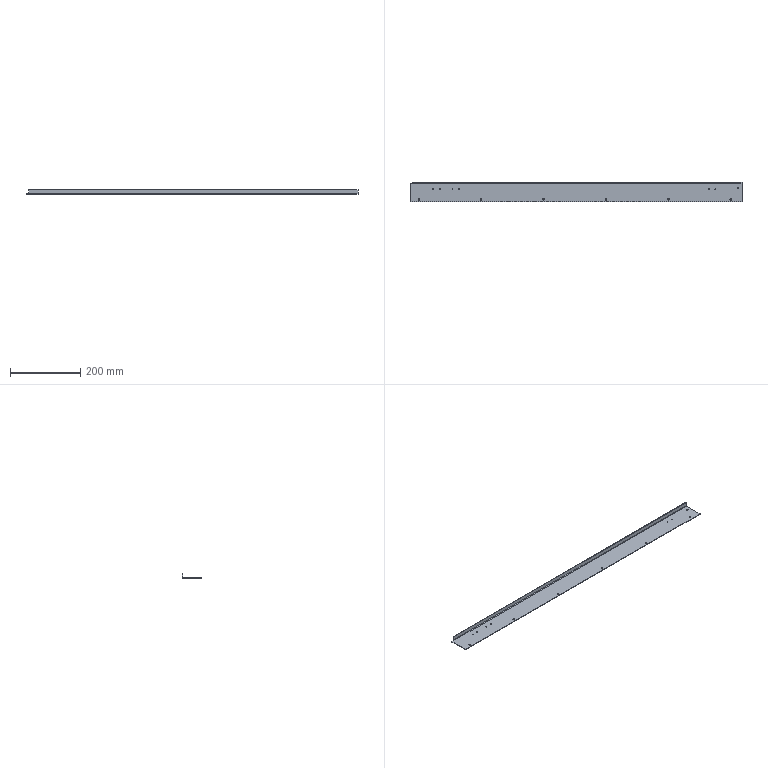Part | STEP file | 866-BDO024-95-04A | 1 solid | 38 faces | box 942 x 56.5 x 13.5 mm | volume 95046 mm3 | cylinder 28 | plane 10 | commonest cylinder face diameters 4.5 x14 2.5 x12 3 x1 6 x1
STEP:
#1=CARTESIAN_POINT('',(730.75,7.5,0.));
#2=VERTEX_POINT('',#1);
#3=CARTESIAN_POINT('',(735.25,7.5,0.));
#4=VERTEX_POINT('',#3);
#5=CARTESIAN_POINT('',(733.,7.5,0.));
#6=DIRECTION('',(0.,0.,1.));
#7=DIRECTION('',(1.,0.,0.));
#8=AXIS2_PLACEMENT_3D('',#5,#6,#7);
#9=CIRCLE('',#8,2.25);
#10=EDGE_CURVE('',#2,#4,#9,.T.);
#11=ORIENTED_EDGE('',*,*,#10,.F.);
#12=CARTESIAN_POINT('',(730.75,7.5,1.5));
#13=VERTEX_POINT('',#12);
#14=CARTESIAN_POINT('',(730.75,7.5,1.5));
#15=DIRECTION('',(0.,0.,1.));
#16=VECTOR('',#15,1000.);
#17=LINE('',#14,#16);
#18=EDGE_CURVE('',#2,#13,#17,.T.);
#19=ORIENTED_EDGE('',*,*,#18,.T.);
#20=CARTESIAN_POINT('',(735.25,7.5,1.5));
#21=VERTEX_POINT('',#20);
#22=CARTESIAN_POINT('',(733.,7.5,1.5));
#23=DIRECTION('',(0.,0.,-1.));
#24=DIRECTION('',(1.,0.,0.));
#25=AXIS2_PLACEMENT_3D('',#22,#23,#24);
#26=CIRCLE('',#25,2.25);
#27=EDGE_CURVE('',#21,#13,#26,.T.);
#28=ORIENTED_EDGE('',*,*,#27,.F.);
#29=CARTESIAN_POINT('',(735.25,7.5,1.5));
#30=DIRECTION('',(0.,0.,1.));
#31=VECTOR('',#30,1000.);
#32=LINE('',#29,#31);
#33=EDGE_CURVE('',#4,#21,#32,.T.);
#34=ORIENTED_EDGE('',*,*,#33,.F.);
#35=EDGE_LOOP('',(#11,#19,#28,#34));
#36=FACE_OUTER_BOUND('',#35,.T.);
#37=CARTESIAN_POINT('',(733.,7.5,1.5));
#38=DIRECTION('',(0.,0.,1.));
#39=DIRECTION('',(1.,0.,0.));
#40=AXIS2_PLACEMENT_3D('',#37,#38,#39);
#41=CYLINDRICAL_SURFACE('',#40,2.25);
#42=ADVANCED_FACE('',(#36),#41,.F.);
#43=CARTESIAN_POINT('',(199.75,7.5,0.));
#44=VERTEX_POINT('',#43);
#45=CARTESIAN_POINT('',(204.25,7.5,0.));
#46=VERTEX_POINT('',#45);
#47=CARTESIAN_POINT('',(202.,7.5,0.));
#48=DIRECTION('',(0.,0.,1.));
#49=DIRECTION('',(1.,0.,0.));
#50=AXIS2_PLACEMENT_3D('',#47,#48,#49);
#51=CIRCLE('',#50,2.25);
#52=EDGE_CURVE('',#44,#46,#51,.T.);
#53=ORIENTED_EDGE('',*,*,#52,.F.);
#54=CARTESIAN_POINT('',(199.75,7.5,1.5));
#55=VERTEX_POINT('',#54);
#56=CARTESIAN_POINT('',(199.75,7.5,1.5));
#57=DIRECTION('',(0.,0.,1.));
#58=VECTOR('',#57,1000.);
#59=LINE('',#56,#58);
#60=EDGE_CURVE('',#44,#55,#59,.T.);
#61=ORIENTED_EDGE('',*,*,#60,.T.);
#62=CARTESIAN_POINT('',(204.25,7.5,1.5));
#63=VERTEX_POINT('',#62);
#64=CARTESIAN_POINT('',(202.,7.5,1.5));
#65=DIRECTION('',(0.,0.,-1.));
#66=DIRECTION('',(1.,0.,0.));
#67=AXIS2_PLACEMENT_3D('',#64,#65,#66);
#68=CIRCLE('',#67,2.25);
#69=EDGE_CURVE('',#63,#55,#68,.T.);
#70=ORIENTED_EDGE('',*,*,#69,.F.);
#71=CARTESIAN_POINT('',(204.25,7.5,1.5));
#72=DIRECTION('',(0.,0.,1.));
#73=VECTOR('',#72,1000.);
#74=LINE('',#71,#73);
#75=EDGE_CURVE('',#46,#63,#74,.T.);
#76=ORIENTED_EDGE('',*,*,#75,.F.);
#77=EDGE_LOOP('',(#53,#61,#70,#76));
#78=FACE_OUTER_BOUND('',#77,.T.);
#79=CARTESIAN_POINT('',(202.,7.5,1.5));
#80=DIRECTION('',(0.,0.,1.));
#81=DIRECTION('',(1.,0.,0.));
#82=AXIS2_PLACEMENT_3D('',#79,#80,#81);
#83=CYLINDRICAL_SURFACE('',#82,2.25);
#84=ADVANCED_FACE('',(#78),#83,.F.);
#85=CARTESIAN_POINT('',(376.75,7.5,0.));
#86=VERTEX_POINT('',#85);
#87=CARTESIAN_POINT('',(381.25,7.5,0.));
#88=VERTEX_POINT('',#87);
#89=CARTESIAN_POINT('',(379.,7.5,0.));
#90=DIRECTION('',(0.,0.,1.));
#91=DIRECTION('',(1.,0.,0.));
#92=AXIS2_PLACEMENT_3D('',#89,#90,#91);
#93=CIRCLE('',#92,2.25);
#94=EDGE_CURVE('',#86,#88,#93,.T.);
#95=ORIENTED_EDGE('',*,*,#94,.F.);
#96=CARTESIAN_POINT('',(376.75,7.5,1.5));
#97=VERTEX_POINT('',#96);
#98=CARTESIAN_POINT('',(376.75,7.5,1.5));
#99=DIRECTION('',(0.,0.,1.));
#100=VECTOR('',#99,1000.);
#101=LINE('',#98,#100);
#102=EDGE_CURVE('',#86,#97,#101,.T.);
#103=ORIENTED_EDGE('',*,*,#102,.T.);
#104=CARTESIAN_POINT('',(381.25,7.5,1.5));
#105=VERTEX_POINT('',#104);
#106=CARTESIAN_POINT('',(379.,7.5,1.5));
#107=DIRECTION('',(0.,0.,-1.));
#108=DIRECTION('',(1.,0.,0.));
#109=AXIS2_PLACEMENT_3D('',#106,#107,#108);
#110=CIRCLE('',#109,2.25);
#111=EDGE_CURVE('',#105,#97,#110,.T.);
#112=ORIENTED_EDGE('',*,*,#111,.F.);
#113=CARTESIAN_POINT('',(381.25,7.5,1.5));
#114=DIRECTION('',(0.,0.,1.));
#115=VECTOR('',#114,1000.);
#116=LINE('',#113,#115);
#117=EDGE_CURVE('',#88,#105,#116,.T.);
#118=ORIENTED_EDGE('',*,*,#117,.F.);
#119=EDGE_LOOP('',(#95,#103,#112,#118));
#120=FACE_OUTER_BOUND('',#119,.T.);
#121=CARTESIAN_POINT('',(379.,7.5,1.5));
#122=DIRECTION('',(0.,0.,1.));
#123=DIRECTION('',(1.,0.,0.));
#124=AXIS2_PLACEMENT_3D('',#121,#122,#123);
#125=CYLINDRICAL_SURFACE('',#124,2.25);
#126=ADVANCED_FACE('',(#120),#125,.F.);
#127=CARTESIAN_POINT('',(553.75,7.5,0.));
#128=VERTEX_POINT('',#127);
#129=CARTESIAN_POINT('',(558.25,7.5,0.));
#130=VERTEX_POINT('',#129);
#131=CARTESIAN_POINT('',(556.,7.5,0.));
#132=DIRECTION('',(0.,0.,1.));
#133=DIRECTION('',(1.,0.,0.));
#134=AXIS2_PLACEMENT_3D('',#131,#132,#133);
#135=CIRCLE('',#134,2.25);
#136=EDGE_CURVE('',#128,#130,#135,.T.);
#137=ORIENTED_EDGE('',*,*,#136,.F.);
#138=CARTESIAN_POINT('',(553.75,7.5,1.5));
#139=VERTEX_POINT('',#138);
#140=CARTESIAN_POINT('',(553.75,7.5,1.5));
#141=DIRECTION('',(0.,0.,1.));
#142=VECTOR('',#141,1000.);
#143=LINE('',#140,#142);
#144=EDGE_CURVE('',#128,#139,#143,.T.);
#145=ORIENTED_EDGE('',*,*,#144,.T.);
#146=CARTESIAN_POINT('',(558.25,7.5,1.5));
#147=VERTEX_POINT('',#146);
#148=CARTESIAN_POINT('',(556.,7.5,1.5));
#149=DIRECTION('',(0.,0.,-1.));
#150=DIRECTION('',(1.,0.,0.));
#151=AXIS2_PLACEMENT_3D('',#148,#149,#150);
#152=CIRCLE('',#151,2.25);
#153=EDGE_CURVE('',#147,#139,#152,.T.);
#154=ORIENTED_EDGE('',*,*,#153,.F.);
#155=CARTESIAN_POINT('',(558.25,7.5,1.5));
#156=DIRECTION('',(0.,0.,1.));
#157=VECTOR('',#156,1000.);
#158=LINE('',#155,#157);
#159=EDGE_CURVE('',#130,#147,#158,.T.);
#160=ORIENTED_EDGE('',*,*,#159,.F.);
#161=EDGE_LOOP('',(#137,#145,#154,#160));
#162=FACE_OUTER_BOUND('',#161,.T.);
#163=CARTESIAN_POINT('',(556.,7.5,1.5));
#164=DIRECTION('',(0.,0.,1.));
#165=DIRECTION('',(1.,0.,0.));
#166=AXIS2_PLACEMENT_3D('',#163,#164,#165);
#167=CYLINDRICAL_SURFACE('',#166,2.25);
#168=ADVANCED_FACE('',(#162),#167,.F.);
#169=CARTESIAN_POINT('',(928.25,40.,0.));
#170=VERTEX_POINT('',#169);
#171=CARTESIAN_POINT('',(932.75,40.,0.));
#172=VERTEX_POINT('',#171);
#173=CARTESIAN_POINT('',(930.5,40.,0.));
#174=DIRECTION('',(0.,0.,1.));
#175=DIRECTION('',(1.,0.,0.));
#176=AXIS2_PLACEMENT_3D('',#173,#174,#175);
#177=CIRCLE('',#176,2.25);
#178=EDGE_CURVE('',#170,#172,#177,.T.);
#179=ORIENTED_EDGE('',*,*,#178,.F.);
#180=CARTESIAN_POINT('',(928.25,40.,1.5));
#181=VERTEX_POINT('',#180);
#182=CARTESIAN_POINT('',(928.25,40.,1.5));
#183=DIRECTION('',(0.,0.,1.));
#184=VECTOR('',#183,1000.);
#185=LINE('',#182,#184);
#186=EDGE_CURVE('',#170,#181,#185,.T.);
#187=ORIENTED_EDGE('',*,*,#186,.T.);
#188=CARTESIAN_POINT('',(932.75,40.,1.5));
#189=VERTEX_POINT('',#188);
#190=CARTESIAN_POINT('',(930.5,40.,1.5));
#191=DIRECTION('',(0.,0.,-1.));
#192=DIRECTION('',(1.,0.,0.));
#193=AXIS2_PLACEMENT_3D('',#190,#191,#192);
#194=CIRCLE('',#193,2.25);
#195=EDGE_CURVE('',#189,#181,#194,.T.);
#196=ORIENTED_EDGE('',*,*,#195,.F.);
#197=CARTESIAN_POINT('',(932.75,40.,1.5));
#198=DIRECTION('',(0.,0.,1.));
#199=VECTOR('',#198,1000.);
#200=LINE('',#197,#199);
#201=EDGE_CURVE('',#172,#189,#200,.T.);
#202=ORIENTED_EDGE('',*,*,#201,.F.);
#203=EDGE_LOOP('',(#179,#187,#196,#202));
#204=FACE_OUTER_BOUND('',#203,.T.);
#205=CARTESIAN_POINT('',(930.5,40.,1.5));
#206=DIRECTION('',(0.,0.,1.));
#207=DIRECTION('',(1.,0.,0.));
#208=AXIS2_PLACEMENT_3D('',#205,#206,#207);
#209=CYLINDRICAL_SURFACE('',#208,2.25);
#210=ADVANCED_FACE('',(#204),#209,.F.);
#211=CARTESIAN_POINT('',(907.75,7.5,0.));
#212=VERTEX_POINT('',#211);
#213=CARTESIAN_POINT('',(912.25,7.5,0.));
#214=VERTEX_POINT('',#213);
#215=CARTESIAN_POINT('',(910.,7.5,0.));
#216=DIRECTION('',(0.,0.,1.));
#217=DIRECTION('',(1.,0.,0.));
#218=AXIS2_PLACEMENT_3D('',#215,#216,#217);
#219=CIRCLE('',#218,2.25);
#220=EDGE_CURVE('',#212,#214,#219,.T.);
#221=ORIENTED_EDGE('',*,*,#220,.F.);
#222=CARTESIAN_POINT('',(907.75,7.5,1.5));
#223=VERTEX_POINT('',#222);
#224=CARTESIAN_POINT('',(907.75,7.5,1.5));
#225=DIRECTION('',(0.,0.,1.));
#226=VECTOR('',#225,1000.);
#227=LINE('',#224,#226);
#228=EDGE_CURVE('',#212,#223,#227,.T.);
#229=ORIENTED_EDGE('',*,*,#228,.T.);
#230=CARTESIAN_POINT('',(912.25,7.5,1.5));
#231=VERTEX_POINT('',#230);
#232=CARTESIAN_POINT('',(910.,7.5,1.5));
#233=DIRECTION('',(0.,0.,-1.));
#234=DIRECTION('',(1.,0.,0.));
#235=AXIS2_PLACEMENT_3D('',#232,#233,#234);
#236=CIRCLE('',#235,2.25);
#237=EDGE_CURVE('',#231,#223,#236,.T.);
#238=ORIENTED_EDGE('',*,*,#237,.F.);
#239=CARTESIAN_POINT('',(912.25,7.5,1.5));
#240=DIRECTION('',(0.,0.,1.));
#241=VECTOR('',#240,1000.);
#242=LINE('',#239,#241);
#243=EDGE_CURVE('',#214,#231,#242,.T.);
#244=ORIENTED_EDGE('',*,*,#243,.F.);
#245=EDGE_LOOP('',(#221,#229,#238,#244));
#246=FACE_OUTER_BOUND('',#245,.T.);
#247=CARTESIAN_POINT('',(910.,7.5,1.5));
#248=DIRECTION('',(0.,0.,1.));
#249=DIRECTION('',(1.,0.,0.));
#250=AXIS2_PLACEMENT_3D('',#247,#248,#249);
#251=CYLINDRICAL_SURFACE('',#250,2.25);
#252=ADVANCED_FACE('',(#246),#251,.F.);
#253=CARTESIAN_POINT('',(22.75,7.5,0.));
#254=VERTEX_POINT('',#253);
#255=CARTESIAN_POINT('',(27.25,7.5,0.));
#256=VERTEX_POINT('',#255);
#257=CARTESIAN_POINT('',(25.,7.5,0.));
#258=DIRECTION('',(0.,0.,1.));
#259=DIRECTION('',(1.,0.,0.));
#260=AXIS2_PLACEMENT_3D('',#257,#258,#259);
#261=CIRCLE('',#260,2.25);
#262=EDGE_CURVE('',#254,#256,#261,.T.);
#263=ORIENTED_EDGE('',*,*,#262,.F.);
#264=CARTESIAN_POINT('',(22.75,7.5,1.5));
#265=VERTEX_POINT('',#264);
#266=CARTESIAN_POINT('',(22.75,7.5,1.5));
#267=DIRECTION('',(0.,0.,1.));
#268=VECTOR('',#267,1000.);
#269=LINE('',#266,#268);
#270=EDGE_CURVE('',#254,#265,#269,.T.);
#271=ORIENTED_EDGE('',*,*,#270,.T.);
#272=CARTESIAN_POINT('',(27.25,7.5,1.5));
#273=VERTEX_POINT('',#272);
#274=CARTESIAN_POINT('',(25.,7.5,1.5));
#275=DIRECTION('',(0.,0.,-1.));
#276=DIRECTION('',(1.,0.,0.));
#277=AXIS2_PLACEMENT_3D('',#274,#275,#276);
#278=CIRCLE('',#277,2.25);
#279=EDGE_CURVE('',#273,#265,#278,.T.);
#280=ORIENTED_EDGE('',*,*,#279,.F.);
#281=CARTESIAN_POINT('',(27.25,7.5,1.5));
#282=DIRECTION('',(0.,0.,1.));
#283=VECTOR('',#282,1000.);
#284=LINE('',#281,#283);
#285=EDGE_CURVE('',#256,#273,#284,.T.);
#286=ORIENTED_EDGE('',*,*,#285,.F.);
#287=EDGE_LOOP('',(#263,#271,#280,#286));
#288=FACE_OUTER_BOUND('',#287,.T.);
#289=CARTESIAN_POINT('',(25.,7.5,1.5));
#290=DIRECTION('',(0.,0.,1.));
#291=DIRECTION('',(1.,0.,0.));
#292=AXIS2_PLACEMENT_3D('',#289,#290,#291);
#293=CYLINDRICAL_SURFACE('',#292,2.25);
#294=ADVANCED_FACE('',(#288),#293,.F.);
#295=CARTESIAN_POINT('',(865.25,36.,0.));
#296=VERTEX_POINT('',#295);
#297=CARTESIAN_POINT('',(867.75,36.,0.));
#298=VERTEX_POINT('',#297);
#299=CARTESIAN_POINT('',(866.5,36.,0.));
#300=DIRECTION('',(0.,0.,1.));
#301=DIRECTION('',(1.,0.,0.));
#302=AXIS2_PLACEMENT_3D('',#299,#300,#301);
#303=CIRCLE('',#302,1.25);
#304=EDGE_CURVE('',#296,#298,#303,.T.);
#305=ORIENTED_EDGE('',*,*,#304,.F.);
#306=CARTESIAN_POINT('',(865.25,36.,1.5));
#307=VERTEX_POINT('',#306);
#308=CARTESIAN_POINT('',(865.25,36.,1.5));
#309=DIRECTION('',(0.,0.,1.));
#310=VECTOR('',#309,1000.);
#311=LINE('',#308,#310);
#312=EDGE_CURVE('',#296,#307,#311,.T.);
#313=ORIENTED_EDGE('',*,*,#312,.T.);
#314=CARTESIAN_POINT('',(867.75,36.,1.5));
#315=VERTEX_POINT('',#314);
#316=CARTESIAN_POINT('',(866.5,36.,1.5));
#317=DIRECTION('',(0.,0.,-1.));
#318=DIRECTION('',(1.,0.,0.));
#319=AXIS2_PLACEMENT_3D('',#316,#317,#318);
#320=CIRCLE('',#319,1.25);
#321=EDGE_CURVE('',#315,#307,#320,.T.);
#322=ORIENTED_EDGE('',*,*,#321,.F.);
#323=CARTESIAN_POINT('',(867.75,36.,1.5));
#324=DIRECTION('',(0.,0.,1.));
#325=VECTOR('',#324,1000.);
#326=LINE('',#323,#325);
#327=EDGE_CURVE('',#298,#315,#326,.T.);
#328=ORIENTED_EDGE('',*,*,#327,.F.);
#329=EDGE_LOOP('',(#305,#313,#322,#328));
#330=FACE_OUTER_BOUND('',#329,.T.);
#331=CARTESIAN_POINT('',(866.5,36.,1.5));
#332=DIRECTION('',(0.,0.,1.));
#333=DIRECTION('',(1.,0.,0.));
#334=AXIS2_PLACEMENT_3D('',#331,#332,#333);
#335=CYLINDRICAL_SURFACE('',#334,1.25);
#336=ADVANCED_FACE('',(#330),#335,.F.);
#337=CARTESIAN_POINT('',(846.25,36.,0.));
#338=VERTEX_POINT('',#337);
#339=CARTESIAN_POINT('',(848.75,36.,0.));
#340=VERTEX_POINT('',#339);
#341=CARTESIAN_POINT('',(847.5,36.,0.));
#342=DIRECTION('',(0.,0.,1.));
#343=DIRECTION('',(1.,0.,0.));
#344=AXIS2_PLACEMENT_3D('',#341,#342,#343);
#345=CIRCLE('',#344,1.25);
#346=EDGE_CURVE('',#338,#340,#345,.T.);
#347=ORIENTED_EDGE('',*,*,#346,.F.);
#348=CARTESIAN_POINT('',(846.25,36.,1.5));
#349=VERTEX_POINT('',#348);
#350=CARTESIAN_POINT('',(846.25,36.,1.5));
#351=DIRECTION('',(0.,0.,1.));
#352=VECTOR('',#351,1000.);
#353=LINE('',#350,#352);
#354=EDGE_CURVE('',#338,#349,#353,.T.);
#355=ORIENTED_EDGE('',*,*,#354,.T.);
#356=CARTESIAN_POINT('',(848.75,36.,1.5));
#357=VERTEX_POINT('',#356);
#358=CARTESIAN_POINT('',(847.5,36.,1.5));
#359=DIRECTION('',(0.,0.,-1.));
#360=DIRECTION('',(1.,0.,0.));
#361=AXIS2_PLACEMENT_3D('',#358,#359,#360);
#362=CIRCLE('',#361,1.25);
#363=EDGE_CURVE('',#357,#349,#362,.T.);
#364=ORIENTED_EDGE('',*,*,#363,.F.);
#365=CARTESIAN_POINT('',(848.75,36.,1.5));
#366=DIRECTION('',(0.,0.,1.));
#367=VECTOR('',#366,1000.);
#368=LINE('',#365,#367);
#369=EDGE_CURVE('',#340,#357,#368,.T.);
#370=ORIENTED_EDGE('',*,*,#369,.F.);
#371=EDGE_LOOP('',(#347,#355,#364,#370));
#372=FACE_OUTER_BOUND('',#371,.T.);
#373=CARTESIAN_POINT('',(847.5,36.,1.5));
#374=DIRECTION('',(0.,0.,1.));
#375=DIRECTION('',(1.,0.,0.));
#376=AXIS2_PLACEMENT_3D('',#373,#374,#375);
#377=CYLINDRICAL_SURFACE('',#376,1.25);
#378=ADVANCED_FACE('',(#372),#377,.F.);
#379=CARTESIAN_POINT('',(138.25,36.,0.));
#380=VERTEX_POINT('',#379);
#381=CARTESIAN_POINT('',(140.75,36.,0.));
#382=VERTEX_POINT('',#381);
#383=CARTESIAN_POINT('',(139.5,36.,0.));
#384=DIRECTION('',(0.,0.,1.));
#385=DIRECTION('',(1.,0.,0.));
#386=AXIS2_PLACEMENT_3D('',#383,#384,#385);
#387=CIRCLE('',#386,1.25);
#388=EDGE_CURVE('',#380,#382,#387,.T.);
#389=ORIENTED_EDGE('',*,*,#388,.F.);
#390=CARTESIAN_POINT('',(138.25,36.,1.5));
#391=VERTEX_POINT('',#390);
#392=CARTESIAN_POINT('',(138.25,36.,1.5));
#393=DIRECTION('',(0.,0.,1.));
#394=VECTOR('',#393,1000.);
#395=LINE('',#392,#394);
#396=EDGE_CURVE('',#380,#391,#395,.T.);
#397=ORIENTED_EDGE('',*,*,#396,.T.);
#398=CARTESIAN_POINT('',(140.75,36.,1.5));
#399=VERTEX_POINT('',#398);
#400=CARTESIAN_POINT('',(139.5,36.,1.5));
#401=DIRECTION('',(0.,0.,-1.));
#402=DIRECTION('',(1.,0.,0.));
#403=AXIS2_PLACEMENT_3D('',#400,#401,#402);
#404=CIRCLE('',#403,1.25);
#405=EDGE_CURVE('',#399,#391,#404,.T.);
#406=ORIENTED_EDGE('',*,*,#405,.F.);
#407=CARTESIAN_POINT('',(140.75,36.,1.5));
#408=DIRECTION('',(0.,0.,1.));
#409=VECTOR('',#408,1000.);
#410=LINE('',#407,#409);
#411=EDGE_CURVE('',#382,#399,#410,.T.);
#412=ORIENTED_EDGE('',*,*,#411,.F.);
#413=EDGE_LOOP('',(#389,#397,#406,#412));
#414=FACE_OUTER_BOUND('',#413,.T.);
#415=CARTESIAN_POINT('',(139.5,36.,1.5));
#416=DIRECTION('',(0.,0.,1.));
#417=DIRECTION('',(1.,0.,0.));
#418=AXIS2_PLACEMENT_3D('',#415,#416,#417);
#419=CYLINDRICAL_SURFACE('',#418,1.25);
#420=ADVANCED_FACE('',(#414),#419,.F.);
#421=CARTESIAN_POINT('',(83.25,36.,0.));
#422=VERTEX_POINT('',#421);
#423=CARTESIAN_POINT('',(85.75,36.,0.));
#424=VERTEX_POINT('',#423);
#425=CARTESIAN_POINT('',(84.5,36.,0.));
#426=DIRECTION('',(0.,0.,1.));
#427=DIRECTION('',(1.,0.,0.));
#428=AXIS2_PLACEMENT_3D('',#425,#426,#427);
#429=CIRCLE('',#428,1.25);
#430=EDGE_CURVE('',#422,#424,#429,.T.);
#431=ORIENTED_EDGE('',*,*,#430,.F.);
#432=CARTESIAN_POINT('',(83.25,36.,1.5));
#433=VERTEX_POINT('',#432);
#434=CARTESIAN_POINT('',(83.25,36.,1.5));
#435=DIRECTION('',(0.,0.,1.));
#436=VECTOR('',#435,1000.);
#437=LINE('',#434,#436);
#438=EDGE_CURVE('',#422,#433,#437,.T.);
#439=ORIENTED_EDGE('',*,*,#438,.T.);
#440=CARTESIAN_POINT('',(85.75,36.,1.5));
#441=VERTEX_POINT('',#440);
#442=CARTESIAN_POINT('',(84.5,36.,1.5));
#443=DIRECTION('',(0.,0.,-1.));
#444=DIRECTION('',(1.,0.,0.));
#445=AXIS2_PLACEMENT_3D('',#442,#443,#444);
#446=CIRCLE('',#445,1.25);
#447=EDGE_CURVE('',#441,#433,#446,.T.);
#448=ORIENTED_EDGE('',*,*,#447,.F.);
#449=CARTESIAN_POINT('',(85.75,36.,1.5));
#450=DIRECTION('',(0.,0.,1.));
#451=VECTOR('',#450,1000.);
#452=LINE('',#449,#451);
#453=EDGE_CURVE('',#424,#441,#452,.T.);
#454=ORIENTED_EDGE('',*,*,#453,.F.);
#455=EDGE_LOOP('',(#431,#439,#448,#454));
#456=FACE_OUTER_BOUND('',#455,.T.);
#457=CARTESIAN_POINT('',(84.5,36.,1.5));
#458=DIRECTION('',(0.,0.,1.));
#459=DIRECTION('',(1.,0.,0.));
#460=AXIS2_PLACEMENT_3D('',#457,#458,#459);
#461=CYLINDRICAL_SURFACE('',#460,1.25);
#462=ADVANCED_FACE('',(#456),#461,.F.);
#463=CARTESIAN_POINT('',(119.25,36.,0.));
#464=VERTEX_POINT('',#463);
#465=CARTESIAN_POINT('',(121.75,36.,0.));
#466=VERTEX_POINT('',#465);
#467=CARTESIAN_POINT('',(120.5,36.,0.));
#468=DIRECTION('',(0.,0.,1.));
#469=DIRECTION('',(1.,0.,0.));
#470=AXIS2_PLACEMENT_3D('',#467,#468,#469);
#471=CIRCLE('',#470,1.25);
#472=EDGE_CURVE('',#464,#466,#471,.T.);
#473=ORIENTED_EDGE('',*,*,#472,.F.);
#474=CARTESIAN_POINT('',(119.25,36.,1.5));
#475=VERTEX_POINT('',#474);
#476=CARTESIAN_POINT('',(119.25,36.,1.5));
#477=DIRECTION('',(0.,0.,1.));
#478=VECTOR('',#477,1000.);
#479=LINE('',#476,#478);
#480=EDGE_CURVE('',#464,#475,#479,.T.);
#481=ORIENTED_EDGE('',*,*,#480,.T.);
#482=CARTESIAN_POINT('',(121.75,36.,1.5));
#483=VERTEX_POINT('',#482);
#484=CARTESIAN_POINT('',(120.5,36.,1.5));
#485=DIRECTION('',(0.,0.,-1.));
#486=DIRECTION('',(1.,0.,0.));
#487=AXIS2_PLACEMENT_3D('',#484,#485,#486);
#488=CIRCLE('',#487,1.25);
#489=EDGE_CURVE('',#483,#475,#488,.T.);
#490=ORIENTED_EDGE('',*,*,#489,.F.);
#491=CARTESIAN_POINT('',(121.75,36.,1.5));
#492=DIRECTION('',(0.,0.,1.));
#493=VECTOR('',#492,1000.);
#494=LINE('',#491,#493);
#495=EDGE_CURVE('',#466,#483,#494,.T.);
#496=ORIENTED_EDGE('',*,*,#495,.F.);
#497=EDGE_LOOP('',(#473,#481,#490,#496));
#498=FACE_OUTER_BOUND('',#497,.T.);
#499=CARTESIAN_POINT('',(120.5,36.,1.5));
#500=DIRECTION('',(0.,0.,1.));
#501=DIRECTION('',(1.,0.,0.));
#502=AXIS2_PLACEMENT_3D('',#499,#500,#501);
#503=CYLINDRICAL_SURFACE('',#502,1.25);
#504=ADVANCED_FACE('',(#498),#503,.F.);
#505=CARTESIAN_POINT('',(64.25,36.,0.));
#506=VERTEX_POINT('',#505);
#507=CARTESIAN_POINT('',(66.75,36.,0.));
#508=VERTEX_POINT('',#507);
#509=CARTESIAN_POINT('',(65.5,36.,0.));
#510=DIRECTION('',(0.,0.,1.));
#511=DIRECTION('',(1.,0.,0.));
#512=AXIS2_PLACEMENT_3D('',#509,#510,#511);
#513=CIRCLE('',#512,1.25);
#514=EDGE_CURVE('',#506,#508,#513,.T.);
#515=ORIENTED_EDGE('',*,*,#514,.F.);
#516=CARTESIAN_POINT('',(64.25,36.,1.5));
#517=VERTEX_POINT('',#516);
#518=CARTESIAN_POINT('',(64.25,36.,1.5));
#519=DIRECTION('',(0.,0.,1.));
#520=VECTOR('',#519,1000.);
#521=LINE('',#518,#520);
#522=EDGE_CURVE('',#506,#517,#521,.T.);
#523=ORIENTED_EDGE('',*,*,#522,.T.);
#524=CARTESIAN_POINT('',(66.75,36.,1.5));
#525=VERTEX_POINT('',#524);
#526=CARTESIAN_POINT('',(65.5,36.,1.5));
#527=DIRECTION('',(0.,0.,-1.));
#528=DIRECTION('',(1.,0.,0.));
#529=AXIS2_PLACEMENT_3D('',#526,#527,#528);
#530=CIRCLE('',#529,1.25);
#531=EDGE_CURVE('',#525,#517,#530,.T.);
#532=ORIENTED_EDGE('',*,*,#531,.F.);
#533=CARTESIAN_POINT('',(66.75,36.,1.5));
#534=DIRECTION('',(0.,0.,1.));
#535=VECTOR('',#534,1000.);
#536=LINE('',#533,#535);
#537=EDGE_CURVE('',#508,#525,#536,.T.);
#538=ORIENTED_EDGE('',*,*,#537,.F.);
#539=EDGE_LOOP('',(#515,#523,#532,#538));
#540=FACE_OUTER_BOUND('',#539,.T.);
#541=CARTESIAN_POINT('',(65.5,36.,1.5));
#542=DIRECTION('',(0.,0.,1.));
#543=DIRECTION('',(1.,0.,0.));
#544=AXIS2_PLACEMENT_3D('',#541,#542,#543);
#545=CYLINDRICAL_SURFACE('',#544,1.25);
#546=ADVANCED_FACE('',(#540),#545,.F.);
#547=CARTESIAN_POINT('',(942.,53.5,1.5));
#548=VERTEX_POINT('',#547);
#549=CARTESIAN_POINT('',(8.,53.5,1.5));
#550=VERTEX_POINT('',#549);
#551=CARTESIAN_POINT('',(942.,53.5,1.5));
#552=DIRECTION('',(-1.,0.,0.));
#553=VECTOR('',#552,1000.);
#554=LINE('',#551,#553);
#555=EDGE_CURVE('',#548,#550,#554,.T.);
#556=ORIENTED_EDGE('',*,*,#555,.T.);
#557=CARTESIAN_POINT('',(0.,53.5,1.5));
#558=VERTEX_POINT('',#557);
#559=CARTESIAN_POINT('',(942.,53.5,1.5));
#560=DIRECTION('',(-1.,0.,0.));
#561=VECTOR('',#560,1000.);
#562=LINE('',#559,#561);
#563=EDGE_CURVE('',#550,#558,#562,.T.);
#564=ORIENTED_EDGE('',*,*,#563,.T.);
#565=CARTESIAN_POINT('',(0.,0.,1.5));
#566=VERTEX_POINT('',#565);
#567=CARTESIAN_POINT('',(0.,0.,1.5));
#568=DIRECTION('',(0.,-1.,0.));
#569=VECTOR('',#568,1000.);
#570=LINE('',#567,#569);
#571=EDGE_CURVE('',#558,#566,#570,.T.);
#572=ORIENTED_EDGE('',*,*,#571,.T.);
#573=CARTESIAN_POINT('',(942.,0.,1.5));
#574=VERTEX_POINT('',#573);
#575=CARTESIAN_POINT('',(942.,0.,1.5));
#576=DIRECTION('',(1.,0.,0.));
#577=VECTOR('',#576,1000.);
#578=LINE('',#575,#577);
#579=EDGE_CURVE('',#566,#574,#578,.T.);
#580=ORIENTED_EDGE('',*,*,#579,.T.);
#581=CARTESIAN_POINT('',(942.,0.,1.5));
#582=DIRECTION('',(0.,1.,0.));
#583=VECTOR('',#582,1000.);
#584=LINE('',#581,#583);
#585=EDGE_CURVE('',#574,#548,#584,.T.);
#586=ORIENTED_EDGE('',*,*,#585,.T.);
#587=EDGE_LOOP('',(#556,#564,#572,#580,#586));
#588=FACE_OUTER_BOUND('',#587,.T.);
#589=ORIENTED_EDGE('',*,*,#27,.T.);
#590=CARTESIAN_POINT('',(733.,7.5,1.5));
#591=DIRECTION('',(0.,0.,-1.));
#592=DIRECTION('',(1.,0.,0.));
#593=AXIS2_PLACEMENT_3D('',#590,#591,#592);
#594=CIRCLE('',#593,2.25);
#595=EDGE_CURVE('',#13,#21,#594,.T.);
#596=ORIENTED_EDGE('',*,*,#595,.T.);
#597=EDGE_LOOP('',(#589,#596));
#598=FACE_BOUND('',#597,.T.);
#599=ORIENTED_EDGE('',*,*,#69,.T.);
#600=CARTESIAN_POINT('',(202.,7.5,1.5));
#601=DIRECTION('',(0.,0.,-1.));
#602=DIRECTION('',(1.,0.,0.));
#603=AXIS2_PLACEMENT_3D('',#600,#601,#602);
#604=CIRCLE('',#603,2.25);
#605=EDGE_CURVE('',#55,#63,#604,.T.);
#606=ORIENTED_EDGE('',*,*,#605,.T.);
#607=EDGE_LOOP('',(#599,#606));
#608=FACE_BOUND('',#607,.T.);
#609=ORIENTED_EDGE('',*,*,#111,.T.);
#610=CARTESIAN_POINT('',(379.,7.5,1.5));
#611=DIRECTION('',(0.,0.,-1.));
#612=DIRECTION('',(1.,0.,0.));
#613=AXIS2_PLACEMENT_3D('',#610,#611,#612);
#614=CIRCLE('',#613,2.25);
#615=EDGE_CURVE('',#97,#105,#614,.T.);
#616=ORIENTED_EDGE('',*,*,#615,.T.);
#617=EDGE_LOOP('',(#609,#616));
#618=FACE_BOUND('',#617,.T.);
#619=ORIENTED_EDGE('',*,*,#153,.T.);
#620=CARTESIAN_POINT('',(556.,7.5,1.5));
#621=DIRECTION('',(0.,0.,-1.));
#622=DIRECTION('',(1.,0.,0.));
#623=AXIS2_PLACEMENT_3D('',#620,#621,#622);
#624=CIRCLE('',#623,2.25);
#625=EDGE_CURVE('',#139,#147,#624,.T.);
#626=ORIENTED_EDGE('',*,*,#625,.T.);
#627=EDGE_LOOP('',(#619,#626));
#628=FACE_BOUND('',#627,.T.);
#629=ORIENTED_EDGE('',*,*,#195,.T.);
#630=CARTESIAN_POINT('',(930.5,40.,1.5));
#631=DIRECTION('',(0.,0.,-1.));
#632=DIRECTION('',(1.,0.,0.));
#633=AXIS2_PLACEMENT_3D('',#630,#631,#632);
#634=CIRCLE('',#633,2.25);
#635=EDGE_CURVE('',#181,#189,#634,.T.);
#636=ORIENTED_EDGE('',*,*,#635,.T.);
#637=EDGE_LOOP('',(#629,#636));
#638=FACE_BOUND('',#637,.T.);
#639=ORIENTED_EDGE('',*,*,#237,.T.);
#640=CARTESIAN_POINT('',(910.,7.5,1.5));
#641=DIRECTION('',(0.,0.,-1.));
#642=DIRECTION('',(1.,0.,0.));
#643=AXIS2_PLACEMENT_3D('',#640,#641,#642);
#644=CIRCLE('',#643,2.25);
#645=EDGE_CURVE('',#223,#231,#644,.T.);
#646=ORIENTED_EDGE('',*,*,#645,.T.);
#647=EDGE_LOOP('',(#639,#646));
#648=FACE_BOUND('',#647,.T.);
#649=ORIENTED_EDGE('',*,*,#279,.T.);
#650=CARTESIAN_POINT('',(25.,7.5,1.5));
#651=DIRECTION('',(0.,0.,-1.));
#652=DIRECTION('',(1.,0.,0.));
#653=AXIS2_PLACEMENT_3D('',#650,#651,#652);
#654=CIRCLE('',#653,2.25);
#655=EDGE_CURVE('',#265,#273,#654,.T.);
#656=ORIENTED_EDGE('',*,*,#655,.T.);
#657=EDGE_LOOP('',(#649,#656));
#658=FACE_BOUND('',#657,.T.);
#659=ORIENTED_EDGE('',*,*,#321,.T.);
#660=CARTESIAN_POINT('',(866.5,36.,1.5));
#661=DIRECTION('',(0.,0.,-1.));
#662=DIRECTION('',(1.,0.,0.));
#663=AXIS2_PLACEMENT_3D('',#660,#661,#662);
#664=CIRCLE('',#663,1.25);
#665=EDGE_CURVE('',#307,#315,#664,.T.);
#666=ORIENTED_EDGE('',*,*,#665,.T.);
#667=EDGE_LOOP('',(#659,#666));
#668=FACE_BOUND('',#667,.T.);
#669=ORIENTED_EDGE('',*,*,#363,.T.);
#670=CARTESIAN_POINT('',(847.5,36.,1.5));
#671=DIRECTION('',(0.,0.,-1.));
#672=DIRECTION('',(1.,0.,0.));
#673=AXIS2_PLACEMENT_3D('',#670,#671,#672);
#674=CIRCLE('',#673,1.25);
#675=EDGE_CURVE('',#349,#357,#674,.T.);
#676=ORIENTED_EDGE('',*,*,#675,.T.);
#677=EDGE_LOOP('',(#669,#676));
#678=FACE_BOUND('',#677,.T.);
#679=ORIENTED_EDGE('',*,*,#405,.T.);
#680=CARTESIAN_POINT('',(139.5,36.,1.5));
#681=DIRECTION('',(0.,0.,-1.));
#682=DIRECTION('',(1.,0.,0.));
#683=AXIS2_PLACEMENT_3D('',#680,#681,#682);
#684=CIRCLE('',#683,1.25);
#685=EDGE_CURVE('',#391,#399,#684,.T.);
#686=ORIENTED_EDGE('',*,*,#685,.T.);
#687=EDGE_LOOP('',(#679,#686));
#688=FACE_BOUND('',#687,.T.);
#689=ORIENTED_EDGE('',*,*,#447,.T.);
#690=CARTESIAN_POINT('',(84.5,36.,1.5));
#691=DIRECTION('',(0.,0.,-1.));
#692=DIRECTION('',(1.,0.,0.));
#693=AXIS2_PLACEMENT_3D('',#690,#691,#692);
#694=CIRCLE('',#693,1.25);
#695=EDGE_CURVE('',#433,#441,#694,.T.);
#696=ORIENTED_EDGE('',*,*,#695,.T.);
#697=EDGE_LOOP('',(#689,#696));
#698=FACE_BOUND('',#697,.T.);
#699=ORIENTED_EDGE('',*,*,#489,.T.);
#700=CARTESIAN_POINT('',(120.5,36.,1.5));
#701=DIRECTION('',(0.,0.,-1.));
#702=DIRECTION('',(1.,0.,0.));
#703=AXIS2_PLACEMENT_3D('',#700,#701,#702);
#704=CIRCLE('',#703,1.25);
#705=EDGE_CURVE('',#475,#483,#704,.T.);
#706=ORIENTED_EDGE('',*,*,#705,.T.);
#707=EDGE_LOOP('',(#699,#706));
#708=FACE_BOUND('',#707,.T.);
#709=ORIENTED_EDGE('',*,*,#531,.T.);
#710=CARTESIAN_POINT('',(65.5,36.,1.5));
#711=DIRECTION('',(0.,0.,-1.));
#712=DIRECTION('',(1.,0.,0.));
#713=AXIS2_PLACEMENT_3D('',#710,#711,#712);
#714=CIRCLE('',#713,1.25);
#715=EDGE_CURVE('',#517,#525,#714,.T.);
#716=ORIENTED_EDGE('',*,*,#715,.T.);
#717=EDGE_LOOP('',(#709,#716));
#718=FACE_BOUND('',#717,.T.);
#719=CARTESIAN_POINT('',(942.,0.,1.5));
#720=DIRECTION('',(0.,0.,1.));
#721=DIRECTION('',(1.,0.,0.));
#722=AXIS2_PLACEMENT_3D('',#719,#720,#721);
#723=PLANE('',#722);
#724=ADVANCED_FACE('',(#588,#598,#608,#618,#628,#638,#648,#658,#668,#678,#688,#698,#708,#718),#723,.T.);
#725=CARTESIAN_POINT('',(8.,53.5,0.));
#726=VERTEX_POINT('',#725);
#727=CARTESIAN_POINT('',(8.,53.5,13.5));
#728=DIRECTION('',(0.,0.,-1.));
#729=VECTOR('',#728,1000.);
#730=LINE('',#727,#729);
#731=EDGE_CURVE('',#550,#726,#730,.T.);
#732=ORIENTED_EDGE('',*,*,#731,.T.);
#733=CARTESIAN_POINT('',(0.,53.5,0.));
#734=VERTEX_POINT('',#733);
#735=CARTESIAN_POINT('',(0.,53.5,0.));
#736=DIRECTION('',(1.,0.,0.));
#737=VECTOR('',#736,1000.);
#738=LINE('',#735,#737);
#739=EDGE_CURVE('',#734,#726,#738,.T.);
#740=ORIENTED_EDGE('',*,*,#739,.F.);
#741=CARTESIAN_POINT('',(0.,53.5,0.));
#742=DIRECTION('',(0.,0.,-1.));
#743=VECTOR('',#742,1000.);
#744=LINE('',#741,#743);
#745=EDGE_CURVE('',#558,#734,#744,.T.);
#746=ORIENTED_EDGE('',*,*,#745,.F.);
#747=ORIENTED_EDGE('',*,*,#563,.F.);
#748=EDGE_LOOP('',(#732,#740,#746,#747));
#749=FACE_OUTER_BOUND('',#748,.T.);
#750=CARTESIAN_POINT('',(0.,53.5,0.));
#751=DIRECTION('',(0.,-1.,0.));
#752=DIRECTION('',(0.,0.,-1.));
#753=AXIS2_PLACEMENT_3D('',#750,#751,#752);
#754=PLANE('',#753);
#755=ADVANCED_FACE('',(#749),#754,.F.);
#756=ORIENTED_EDGE('',*,*,#555,.F.);
#757=CARTESIAN_POINT('',(942.,55.,3.));
#758=VERTEX_POINT('',#757);
#759=CARTESIAN_POINT('',(942.,53.5,3.));
#760=DIRECTION('',(-1.,0.,0.));
#761=DIRECTION('',(0.,0.,1.));
#762=AXIS2_PLACEMENT_3D('',#759,#760,#761);
#763=CIRCLE('',#762,1.5);
#764=EDGE_CURVE('',#758,#548,#763,.T.);
#765=ORIENTED_EDGE('',*,*,#764,.F.);
#766=CARTESIAN_POINT('',(8.,55.,3.));
#767=VERTEX_POINT('',#766);
#768=CARTESIAN_POINT('',(942.,55.,3.));
#769=DIRECTION('',(1.,0.,0.));
#770=VECTOR('',#769,1000.);
#771=LINE('',#768,#770);
#772=EDGE_CURVE('',#767,#758,#771,.T.);
#773=ORIENTED_EDGE('',*,*,#772,.F.);
#774=CARTESIAN_POINT('',(8.,53.5,3.));
#775=DIRECTION('',(1.,0.,0.));
#776=DIRECTION('',(0.,0.,1.));
#777=AXIS2_PLACEMENT_3D('',#774,#775,#776);
#778=CIRCLE('',#777,1.5);
#779=EDGE_CURVE('',#550,#767,#778,.T.);
#780=ORIENTED_EDGE('',*,*,#779,.F.);
#781=EDGE_LOOP('',(#756,#765,#773,#780));
#782=FACE_OUTER_BOUND('',#781,.T.);
#783=CARTESIAN_POINT('',(942.,53.5,3.));
#784=DIRECTION('',(-1.,0.,0.));
#785=DIRECTION('',(0.,0.,1.));
#786=AXIS2_PLACEMENT_3D('',#783,#784,#785);
#787=CYLINDRICAL_SURFACE('',#786,1.5);
#788=ADVANCED_FACE('',(#782),#787,.F.);
#789=ORIENTED_EDGE('',*,*,#585,.F.);
#790=CARTESIAN_POINT('',(942.,0.,0.));
#791=VERTEX_POINT('',#790);
#792=CARTESIAN_POINT('',(942.,0.,3.));
#793=DIRECTION('',(0.,0.,-1.));
#794=VECTOR('',#793,1000.);
#795=LINE('',#792,#794);
#796=EDGE_CURVE('',#574,#791,#795,.T.);
#797=ORIENTED_EDGE('',*,*,#796,.T.);
#798=CARTESIAN_POINT('',(942.,53.5,0.));
#799=VERTEX_POINT('',#798);
#800=CARTESIAN_POINT('',(942.,55.,0.));
#801=DIRECTION('',(0.,1.,0.));
#802=VECTOR('',#801,1000.);
#803=LINE('',#800,#802);
#804=EDGE_CURVE('',#791,#799,#803,.T.);
#805=ORIENTED_EDGE('',*,*,#804,.T.);
#806=CARTESIAN_POINT('',(942.,56.5,3.));
#807=VERTEX_POINT('',#806);
#808=CARTESIAN_POINT('',(942.,53.5,3.));
#809=DIRECTION('',(1.,0.,0.));
#810=DIRECTION('',(0.,0.,1.));
#811=AXIS2_PLACEMENT_3D('',#808,#809,#810);
#812=CIRCLE('',#811,3.);
#813=EDGE_CURVE('',#799,#807,#812,.T.);
#814=ORIENTED_EDGE('',*,*,#813,.T.);
#815=CARTESIAN_POINT('',(942.,56.5,13.5));
#816=VERTEX_POINT('',#815);
#817=CARTESIAN_POINT('',(942.,56.5,0.));
#818=DIRECTION('',(0.,0.,1.));
#819=VECTOR('',#818,1000.);
#820=LINE('',#817,#819);
#821=EDGE_CURVE('',#807,#816,#820,.T.);
#822=ORIENTED_EDGE('',*,*,#821,.T.);
#823=CARTESIAN_POINT('',(942.,55.,13.5));
#824=VERTEX_POINT('',#823);
#825=CARTESIAN_POINT('',(942.,55.,13.5));
#826=DIRECTION('',(0.,1.,0.));
#827=VECTOR('',#826,1000.);
#828=LINE('',#825,#827);
#829=EDGE_CURVE('',#824,#816,#828,.T.);
#830=ORIENTED_EDGE('',*,*,#829,.F.);
#831=CARTESIAN_POINT('',(942.,55.,0.));
#832=DIRECTION('',(0.,0.,1.));
#833=VECTOR('',#832,1000.);
#834=LINE('',#831,#833);
#835=EDGE_CURVE('',#758,#824,#834,.T.);
#836=ORIENTED_EDGE('',*,*,#835,.F.);
#837=ORIENTED_EDGE('',*,*,#764,.T.);
#838=EDGE_LOOP('',(#789,#797,#805,#814,#822,#830,#836,#837));
#839=FACE_OUTER_BOUND('',#838,.T.);
#840=CARTESIAN_POINT('',(942.,55.,3.));
#841=DIRECTION('',(1.,0.,0.));
#842=DIRECTION('',(0.,0.,-1.));
#843=AXIS2_PLACEMENT_3D('',#840,#841,#842);
#844=PLANE('',#843);
#845=ADVANCED_FACE('',(#839),#844,.T.);
#846=ORIENTED_EDGE('',*,*,#796,.F.);
#847=ORIENTED_EDGE('',*,*,#579,.F.);
#848=CARTESIAN_POINT('',(0.,0.,0.));
#849=VERTEX_POINT('',#848);
#850=CARTESIAN_POINT('',(0.,0.,0.));
#851=DIRECTION('',(0.,0.,-1.));
#852=VECTOR('',#851,1000.);
#853=LINE('',#850,#852);
#854=EDGE_CURVE('',#566,#849,#853,.T.);
#855=ORIENTED_EDGE('',*,*,#854,.T.);
#856=CARTESIAN_POINT('',(942.,0.,0.));
#857=DIRECTION('',(1.,0.,0.));
#858=VECTOR('',#857,1000.);
#859=LINE('',#856,#858);
#860=EDGE_CURVE('',#849,#791,#859,.T.);
#861=ORIENTED_EDGE('',*,*,#860,.T.);
#862=EDGE_LOOP('',(#846,#847,#855,#861));
#863=FACE_OUTER_BOUND('',#862,.T.);
#864=CARTESIAN_POINT('',(942.,0.,0.));
#865=DIRECTION('',(0.,-1.,0.));
#866=DIRECTION('',(0.,0.,-1.));
#867=AXIS2_PLACEMENT_3D('',#864,#865,#866);
#868=PLANE('',#867);
#869=ADVANCED_FACE('',(#863),#868,.T.);
#870=ORIENTED_EDGE('',*,*,#745,.T.);
#871=CARTESIAN_POINT('',(0.,53.5,0.));
#872=DIRECTION('',(0.,1.,0.));
#873=VECTOR('',#872,1000.);
#874=LINE('',#871,#873);
#875=EDGE_CURVE('',#849,#734,#874,.T.);
#876=ORIENTED_EDGE('',*,*,#875,.F.);
#877=ORIENTED_EDGE('',*,*,#854,.F.);
#878=ORIENTED_EDGE('',*,*,#571,.F.);
#879=EDGE_LOOP('',(#870,#876,#877,#878));
#880=FACE_OUTER_BOUND('',#879,.T.);
#881=CARTESIAN_POINT('',(0.,53.5,3.));
#882=DIRECTION('',(1.,0.,0.));
#883=DIRECTION('',(0.,0.,-1.));
#884=AXIS2_PLACEMENT_3D('',#881,#882,#883);
#885=PLANE('',#884);
#886=ADVANCED_FACE('',(#880),#885,.F.);
#887=ORIENTED_EDGE('',*,*,#18,.F.);
#888=CARTESIAN_POINT('',(733.,7.5,0.));
#889=DIRECTION('',(0.,0.,1.));
#890=DIRECTION('',(1.,0.,0.));
#891=AXIS2_PLACEMENT_3D('',#888,#889,#890);
#892=CIRCLE('',#891,2.25);
#893=EDGE_CURVE('',#4,#2,#892,.T.);
#894=ORIENTED_EDGE('',*,*,#893,.F.);
#895=ORIENTED_EDGE('',*,*,#33,.T.);
#896=ORIENTED_EDGE('',*,*,#595,.F.);
#897=EDGE_LOOP('',(#887,#894,#895,#896));
#898=FACE_OUTER_BOUND('',#897,.T.);
#899=CARTESIAN_POINT('',(733.,7.5,1.5));
#900=DIRECTION('',(0.,0.,1.));
#901=DIRECTION('',(1.,0.,0.));
#902=AXIS2_PLACEMENT_3D('',#899,#900,#901);
#903=CYLINDRICAL_SURFACE('',#902,2.25);
#904=ADVANCED_FACE('',(#898),#903,.F.);
#905=ORIENTED_EDGE('',*,*,#60,.F.);
#906=CARTESIAN_POINT('',(202.,7.5,0.));
#907=DIRECTION('',(0.,0.,1.));
#908=DIRECTION('',(1.,0.,0.));
#909=AXIS2_PLACEMENT_3D('',#906,#907,#908);
#910=CIRCLE('',#909,2.25);
#911=EDGE_CURVE('',#46,#44,#910,.T.);
#912=ORIENTED_EDGE('',*,*,#911,.F.);
#913=ORIENTED_EDGE('',*,*,#75,.T.);
#914=ORIENTED_EDGE('',*,*,#605,.F.);
#915=EDGE_LOOP('',(#905,#912,#913,#914));
#916=FACE_OUTER_BOUND('',#915,.T.);
#917=CARTESIAN_POINT('',(202.,7.5,1.5));
#918=DIRECTION('',(0.,0.,1.));
#919=DIRECTION('',(1.,0.,0.));
#920=AXIS2_PLACEMENT_3D('',#917,#918,#919);
#921=CYLINDRICAL_SURFACE('',#920,2.25);
#922=ADVANCED_FACE('',(#916),#921,.F.);
#923=ORIENTED_EDGE('',*,*,#102,.F.);
#924=CARTESIAN_POINT('',(379.,7.5,0.));
#925=DIRECTION('',(0.,0.,1.));
#926=DIRECTION('',(1.,0.,0.));
#927=AXIS2_PLACEMENT_3D('',#924,#925,#926);
#928=CIRCLE('',#927,2.25);
#929=EDGE_CURVE('',#88,#86,#928,.T.);
#930=ORIENTED_EDGE('',*,*,#929,.F.);
#931=ORIENTED_EDGE('',*,*,#117,.T.);
#932=ORIENTED_EDGE('',*,*,#615,.F.);
#933=EDGE_LOOP('',(#923,#930,#931,#932));
#934=FACE_OUTER_BOUND('',#933,.T.);
#935=CARTESIAN_POINT('',(379.,7.5,1.5));
#936=DIRECTION('',(0.,0.,1.));
#937=DIRECTION('',(1.,0.,0.));
#938=AXIS2_PLACEMENT_3D('',#935,#936,#937);
#939=CYLINDRICAL_SURFACE('',#938,2.25);
#940=ADVANCED_FACE('',(#934),#939,.F.);
#941=ORIENTED_EDGE('',*,*,#144,.F.);
#942=CARTESIAN_POINT('',(556.,7.5,0.));
#943=DIRECTION('',(0.,0.,1.));
#944=DIRECTION('',(1.,0.,0.));
#945=AXIS2_PLACEMENT_3D('',#942,#943,#944);
#946=CIRCLE('',#945,2.25);
#947=EDGE_CURVE('',#130,#128,#946,.T.);
#948=ORIENTED_EDGE('',*,*,#947,.F.);
#949=ORIENTED_EDGE('',*,*,#159,.T.);
#950=ORIENTED_EDGE('',*,*,#625,.F.);
#951=EDGE_LOOP('',(#941,#948,#949,#950));
#952=FACE_OUTER_BOUND('',#951,.T.);
#953=CARTESIAN_POINT('',(556.,7.5,1.5));
#954=DIRECTION('',(0.,0.,1.));
#955=DIRECTION('',(1.,0.,0.));
#956=AXIS2_PLACEMENT_3D('',#953,#954,#955);
#957=CYLINDRICAL_SURFACE('',#956,2.25);
#958=ADVANCED_FACE('',(#952),#957,.F.);
#959=ORIENTED_EDGE('',*,*,#186,.F.);
#960=CARTESIAN_POINT('',(930.5,40.,0.));
#961=DIRECTION('',(0.,0.,1.));
#962=DIRECTION('',(1.,0.,0.));
#963=AXIS2_PLACEMENT_3D('',#960,#961,#962);
#964=CIRCLE('',#963,2.25);
#965=EDGE_CURVE('',#172,#170,#964,.T.);
#966=ORIENTED_EDGE('',*,*,#965,.F.);
#967=ORIENTED_EDGE('',*,*,#201,.T.);
#968=ORIENTED_EDGE('',*,*,#635,.F.);
#969=EDGE_LOOP('',(#959,#966,#967,#968));
#970=FACE_OUTER_BOUND('',#969,.T.);
#971=CARTESIAN_POINT('',(930.5,40.,1.5));
#972=DIRECTION('',(0.,0.,1.));
#973=DIRECTION('',(1.,0.,0.));
#974=AXIS2_PLACEMENT_3D('',#971,#972,#973);
#975=CYLINDRICAL_SURFACE('',#974,2.25);
#976=ADVANCED_FACE('',(#970),#975,.F.);
#977=ORIENTED_EDGE('',*,*,#228,.F.);
#978=CARTESIAN_POINT('',(910.,7.5,0.));
#979=DIRECTION('',(0.,0.,1.));
#980=DIRECTION('',(1.,0.,0.));
#981=AXIS2_PLACEMENT_3D('',#978,#979,#980);
#982=CIRCLE('',#981,2.25);
#983=EDGE_CURVE('',#214,#212,#982,.T.);
#984=ORIENTED_EDGE('',*,*,#983,.F.);
#985=ORIENTED_EDGE('',*,*,#243,.T.);
#986=ORIENTED_EDGE('',*,*,#645,.F.);
#987=EDGE_LOOP('',(#977,#984,#985,#986));
#988=FACE_OUTER_BOUND('',#987,.T.);
#989=CARTESIAN_POINT('',(910.,7.5,1.5));
#990=DIRECTION('',(0.,0.,1.));
#991=DIRECTION('',(1.,0.,0.));
#992=AXIS2_PLACEMENT_3D('',#989,#990,#991);
#993=CYLINDRICAL_SURFACE('',#992,2.25);
#994=ADVANCED_FACE('',(#988),#993,.F.);
#995=ORIENTED_EDGE('',*,*,#270,.F.);
#996=CARTESIAN_POINT('',(25.,7.5,0.));
#997=DIRECTION('',(0.,0.,1.));
#998=DIRECTION('',(1.,0.,0.));
#999=AXIS2_PLACEMENT_3D('',#996,#997,#998);
#1000=CIRCLE('',#999,2.25);
#1001=EDGE_CURVE('',#256,#254,#1000,.T.);
#1002=ORIENTED_EDGE('',*,*,#1001,.F.);
#1003=ORIENTED_EDGE('',*,*,#285,.T.);
#1004=ORIENTED_EDGE('',*,*,#655,.F.);
#1005=EDGE_LOOP('',(#995,#1002,#1003,#1004));
#1006=FACE_OUTER_BOUND('',#1005,.T.);
#1007=CARTESIAN_POINT('',(25.,7.5,1.5));
#1008=DIRECTION('',(0.,0.,1.));
#1009=DIRECTION('',(1.,0.,0.));
#1010=AXIS2_PLACEMENT_3D('',#1007,#1008,#1009);
#1011=CYLINDRICAL_SURFACE('',#1010,2.25);
#1012=ADVANCED_FACE('',(#1006),#1011,.F.);
#1013=ORIENTED_EDGE('',*,*,#312,.F.);
#1014=CARTESIAN_POINT('',(866.5,36.,0.));
#1015=DIRECTION('',(0.,0.,1.));
#1016=DIRECTION('',(1.,0.,0.));
#1017=AXIS2_PLACEMENT_3D('',#1014,#1015,#1016);
#1018=CIRCLE('',#1017,1.25);
#1019=EDGE_CURVE('',#298,#296,#1018,.T.);
#1020=ORIENTED_EDGE('',*,*,#1019,.F.);
#1021=ORIENTED_EDGE('',*,*,#327,.T.);
#1022=ORIENTED_EDGE('',*,*,#665,.F.);
#1023=EDGE_LOOP('',(#1013,#1020,#1021,#1022));
#1024=FACE_OUTER_BOUND('',#1023,.T.);
#1025=CARTESIAN_POINT('',(866.5,36.,1.5));
#1026=DIRECTION('',(0.,0.,1.));
#1027=DIRECTION('',(1.,0.,0.));
#1028=AXIS2_PLACEMENT_3D('',#1025,#1026,#1027);
#1029=CYLINDRICAL_SURFACE('',#1028,1.25);
#1030=ADVANCED_FACE('',(#1024),#1029,.F.);
#1031=ORIENTED_EDGE('',*,*,#354,.F.);
#1032=CARTESIAN_POINT('',(847.5,36.,0.));
#1033=DIRECTION('',(0.,0.,1.));
#1034=DIRECTION('',(1.,0.,0.));
#1035=AXIS2_PLACEMENT_3D('',#1032,#1033,#1034);
#1036=CIRCLE('',#1035,1.25);
#1037=EDGE_CURVE('',#340,#338,#1036,.T.);
#1038=ORIENTED_EDGE('',*,*,#1037,.F.);
#1039=ORIENTED_EDGE('',*,*,#369,.T.);
#1040=ORIENTED_EDGE('',*,*,#675,.F.);
#1041=EDGE_LOOP('',(#1031,#1038,#1039,#1040));
#1042=FACE_OUTER_BOUND('',#1041,.T.);
#1043=CARTESIAN_POINT('',(847.5,36.,1.5));
#1044=DIRECTION('',(0.,0.,1.));
#1045=DIRECTION('',(1.,0.,0.));
#1046=AXIS2_PLACEMENT_3D('',#1043,#1044,#1045);
#1047=CYLINDRICAL_SURFACE('',#1046,1.25);
#1048=ADVANCED_FACE('',(#1042),#1047,.F.);
#1049=ORIENTED_EDGE('',*,*,#396,.F.);
#1050=CARTESIAN_POINT('',(139.5,36.,0.));
#1051=DIRECTION('',(0.,0.,1.));
#1052=DIRECTION('',(1.,0.,0.));
#1053=AXIS2_PLACEMENT_3D('',#1050,#1051,#1052);
#1054=CIRCLE('',#1053,1.25);
#1055=EDGE_CURVE('',#382,#380,#1054,.T.);
#1056=ORIENTED_EDGE('',*,*,#1055,.F.);
#1057=ORIENTED_EDGE('',*,*,#411,.T.);
#1058=ORIENTED_EDGE('',*,*,#685,.F.);
#1059=EDGE_LOOP('',(#1049,#1056,#1057,#1058));
#1060=FACE_OUTER_BOUND('',#1059,.T.);
#1061=CARTESIAN_POINT('',(139.5,36.,1.5));
#1062=DIRECTION('',(0.,0.,1.));
#1063=DIRECTION('',(1.,0.,0.));
#1064=AXIS2_PLACEMENT_3D('',#1061,#1062,#1063);
#1065=CYLINDRICAL_SURFACE('',#1064,1.25);
#1066=ADVANCED_FACE('',(#1060),#1065,.F.);
#1067=ORIENTED_EDGE('',*,*,#438,.F.);
#1068=CARTESIAN_POINT('',(84.5,36.,0.));
#1069=DIRECTION('',(0.,0.,1.));
#1070=DIRECTION('',(1.,0.,0.));
#1071=AXIS2_PLACEMENT_3D('',#1068,#1069,#1070);
#1072=CIRCLE('',#1071,1.25);
#1073=EDGE_CURVE('',#424,#422,#1072,.T.);
#1074=ORIENTED_EDGE('',*,*,#1073,.F.);
#1075=ORIENTED_EDGE('',*,*,#453,.T.);
#1076=ORIENTED_EDGE('',*,*,#695,.F.);
#1077=EDGE_LOOP('',(#1067,#1074,#1075,#1076));
#1078=FACE_OUTER_BOUND('',#1077,.T.);
#1079=CARTESIAN_POINT('',(84.5,36.,1.5));
#1080=DIRECTION('',(0.,0.,1.));
#1081=DIRECTION('',(1.,0.,0.));
#1082=AXIS2_PLACEMENT_3D('',#1079,#1080,#1081);
#1083=CYLINDRICAL_SURFACE('',#1082,1.25);
#1084=ADVANCED_FACE('',(#1078),#1083,.F.);
#1085=ORIENTED_EDGE('',*,*,#480,.F.);
#1086=CARTESIAN_POINT('',(120.5,36.,0.));
#1087=DIRECTION('',(0.,0.,1.));
#1088=DIRECTION('',(1.,0.,0.));
#1089=AXIS2_PLACEMENT_3D('',#1086,#1087,#1088);
#1090=CIRCLE('',#1089,1.25);
#1091=EDGE_CURVE('',#466,#464,#1090,.T.);
#1092=ORIENTED_EDGE('',*,*,#1091,.F.);
#1093=ORIENTED_EDGE('',*,*,#495,.T.);
#1094=ORIENTED_EDGE('',*,*,#705,.F.);
#1095=EDGE_LOOP('',(#1085,#1092,#1093,#1094));
#1096=FACE_OUTER_BOUND('',#1095,.T.);
#1097=CARTESIAN_POINT('',(120.5,36.,1.5));
#1098=DIRECTION('',(0.,0.,1.));
#1099=DIRECTION('',(1.,0.,0.));
#1100=AXIS2_PLACEMENT_3D('',#1097,#1098,#1099);
#1101=CYLINDRICAL_SURFACE('',#1100,1.25);
#1102=ADVANCED_FACE('',(#1096),#1101,.F.);
#1103=ORIENTED_EDGE('',*,*,#522,.F.);
#1104=CARTESIAN_POINT('',(65.5,36.,0.));
#1105=DIRECTION('',(0.,0.,1.));
#1106=DIRECTION('',(1.,0.,0.));
#1107=AXIS2_PLACEMENT_3D('',#1104,#1105,#1106);
#1108=CIRCLE('',#1107,1.25);
#1109=EDGE_CURVE('',#508,#506,#1108,.T.);
#1110=ORIENTED_EDGE('',*,*,#1109,.F.);
#1111=ORIENTED_EDGE('',*,*,#537,.T.);
#1112=ORIENTED_EDGE('',*,*,#715,.F.);
#1113=EDGE_LOOP('',(#1103,#1110,#1111,#1112));
#1114=FACE_OUTER_BOUND('',#1113,.T.);
#1115=CARTESIAN_POINT('',(65.5,36.,1.5));
#1116=DIRECTION('',(0.,0.,1.));
#1117=DIRECTION('',(1.,0.,0.));
#1118=AXIS2_PLACEMENT_3D('',#1115,#1116,#1117);
#1119=CYLINDRICAL_SURFACE('',#1118,1.25);
#1120=ADVANCED_FACE('',(#1114),#1119,.F.);
#1121=ORIENTED_EDGE('',*,*,#739,.T.);
#1122=CARTESIAN_POINT('',(942.,53.5,0.));
#1123=DIRECTION('',(-1.,0.,0.));
#1124=VECTOR('',#1123,1000.);
#1125=LINE('',#1122,#1124);
#1126=EDGE_CURVE('',#799,#726,#1125,.T.);
#1127=ORIENTED_EDGE('',*,*,#1126,.F.);
#1128=ORIENTED_EDGE('',*,*,#804,.F.);
#1129=ORIENTED_EDGE('',*,*,#860,.F.);
#1130=ORIENTED_EDGE('',*,*,#875,.T.);
#1131=EDGE_LOOP('',(#1121,#1127,#1128,#1129,#1130));
#1132=FACE_OUTER_BOUND('',#1131,.T.);
#1133=ORIENTED_EDGE('',*,*,#893,.T.);
#1134=ORIENTED_EDGE('',*,*,#10,.T.);
#1135=EDGE_LOOP('',(#1133,#1134));
#1136=FACE_BOUND('',#1135,.T.);
#1137=ORIENTED_EDGE('',*,*,#911,.T.);
#1138=ORIENTED_EDGE('',*,*,#52,.T.);
#1139=EDGE_LOOP('',(#1137,#1138));
#1140=FACE_BOUND('',#1139,.T.);
#1141=ORIENTED_EDGE('',*,*,#929,.T.);
#1142=ORIENTED_EDGE('',*,*,#94,.T.);
#1143=EDGE_LOOP('',(#1141,#1142));
#1144=FACE_BOUND('',#1143,.T.);
#1145=ORIENTED_EDGE('',*,*,#947,.T.);
#1146=ORIENTED_EDGE('',*,*,#136,.T.);
#1147=EDGE_LOOP('',(#1145,#1146));
#1148=FACE_BOUND('',#1147,.T.);
#1149=ORIENTED_EDGE('',*,*,#965,.T.);
#1150=ORIENTED_EDGE('',*,*,#178,.T.);
#1151=EDGE_LOOP('',(#1149,#1150));
#1152=FACE_BOUND('',#1151,.T.);
#1153=ORIENTED_EDGE('',*,*,#983,.T.);
#1154=ORIENTED_EDGE('',*,*,#220,.T.);
#1155=EDGE_LOOP('',(#1153,#1154));
#1156=FACE_BOUND('',#1155,.T.);
#1157=ORIENTED_EDGE('',*,*,#1001,.T.);
#1158=ORIENTED_EDGE('',*,*,#262,.T.);
#1159=EDGE_LOOP('',(#1157,#1158));
#1160=FACE_BOUND('',#1159,.T.);
#1161=ORIENTED_EDGE('',*,*,#1019,.T.);
#1162=ORIENTED_EDGE('',*,*,#304,.T.);
#1163=EDGE_LOOP('',(#1161,#1162));
#1164=FACE_BOUND('',#1163,.T.);
#1165=ORIENTED_EDGE('',*,*,#1037,.T.);
#1166=ORIENTED_EDGE('',*,*,#346,.T.);
#1167=EDGE_LOOP('',(#1165,#1166));
#1168=FACE_BOUND('',#1167,.T.);
#1169=ORIENTED_EDGE('',*,*,#1055,.T.);
#1170=ORIENTED_EDGE('',*,*,#388,.T.);
#1171=EDGE_LOOP('',(#1169,#1170));
#1172=FACE_BOUND('',#1171,.T.);
#1173=ORIENTED_EDGE('',*,*,#1073,.T.);
#1174=ORIENTED_EDGE('',*,*,#430,.T.);
#1175=EDGE_LOOP('',(#1173,#1174));
#1176=FACE_BOUND('',#1175,.T.);
#1177=ORIENTED_EDGE('',*,*,#1091,.T.);
#1178=ORIENTED_EDGE('',*,*,#472,.T.);
#1179=EDGE_LOOP('',(#1177,#1178));
#1180=FACE_BOUND('',#1179,.T.);
#1181=ORIENTED_EDGE('',*,*,#1109,.T.);
#1182=ORIENTED_EDGE('',*,*,#514,.T.);
#1183=EDGE_LOOP('',(#1181,#1182));
#1184=FACE_BOUND('',#1183,.T.);
#1185=CARTESIAN_POINT('',(942.,0.,0.));
#1186=DIRECTION('',(0.,0.,1.));
#1187=DIRECTION('',(1.,0.,0.));
#1188=AXIS2_PLACEMENT_3D('',#1185,#1186,#1187);
#1189=PLANE('',#1188);
#1190=ADVANCED_FACE('',(#1132,#1136,#1140,#1144,#1148,#1152,#1156,#1160,#1164,#1168,#1172,#1176,#1180,#1184),#1189,.F.);
#1191=CARTESIAN_POINT('',(8.,56.5,13.5));
#1192=VERTEX_POINT('',#1191);
#1193=CARTESIAN_POINT('',(8.,55.,13.5));
#1194=VERTEX_POINT('',#1193);
#1195=CARTESIAN_POINT('',(8.,55.,13.5));
#1196=DIRECTION('',(0.,-1.,0.));
#1197=VECTOR('',#1196,1000.);
#1198=LINE('',#1195,#1197);
#1199=EDGE_CURVE('',#1192,#1194,#1198,.T.);
#1200=ORIENTED_EDGE('',*,*,#1199,.F.);
#1201=CARTESIAN_POINT('',(8.,56.5,3.));
#1202=VERTEX_POINT('',#1201);
#1203=CARTESIAN_POINT('',(8.,56.5,13.5));
#1204=DIRECTION('',(0.,0.,1.));
#1205=VECTOR('',#1204,1000.);
#1206=LINE('',#1203,#1205);
#1207=EDGE_CURVE('',#1202,#1192,#1206,.T.);
#1208=ORIENTED_EDGE('',*,*,#1207,.F.);
#1209=CARTESIAN_POINT('',(8.,53.5,3.));
#1210=DIRECTION('',(1.,0.,0.));
#1211=DIRECTION('',(0.,0.,1.));
#1212=AXIS2_PLACEMENT_3D('',#1209,#1210,#1211);
#1213=CIRCLE('',#1212,3.);
#1214=EDGE_CURVE('',#726,#1202,#1213,.T.);
#1215=ORIENTED_EDGE('',*,*,#1214,.F.);
#1216=ORIENTED_EDGE('',*,*,#731,.F.);
#1217=ORIENTED_EDGE('',*,*,#779,.T.);
#1218=CARTESIAN_POINT('',(8.,55.,13.5));
#1219=DIRECTION('',(0.,0.,-1.));
#1220=VECTOR('',#1219,1000.);
#1221=LINE('',#1218,#1220);
#1222=EDGE_CURVE('',#1194,#767,#1221,.T.);
#1223=ORIENTED_EDGE('',*,*,#1222,.F.);
#1224=EDGE_LOOP('',(#1200,#1208,#1215,#1216,#1217,#1223));
#1225=FACE_OUTER_BOUND('',#1224,.T.);
#1226=CARTESIAN_POINT('',(8.,53.5,13.5));
#1227=DIRECTION('',(1.,0.,0.));
#1228=DIRECTION('',(0.,0.,-1.));
#1229=AXIS2_PLACEMENT_3D('',#1226,#1227,#1228);
#1230=PLANE('',#1229);
#1231=ADVANCED_FACE('',(#1225),#1230,.F.);
#1232=ORIENTED_EDGE('',*,*,#835,.T.);
#1233=CARTESIAN_POINT('',(942.,55.,13.5));
#1234=DIRECTION('',(-1.,0.,0.));
#1235=VECTOR('',#1234,1000.);
#1236=LINE('',#1233,#1235);
#1237=EDGE_CURVE('',#824,#1194,#1236,.T.);
#1238=ORIENTED_EDGE('',*,*,#1237,.T.);
#1239=ORIENTED_EDGE('',*,*,#1222,.T.);
#1240=ORIENTED_EDGE('',*,*,#772,.T.);
#1241=EDGE_LOOP('',(#1232,#1238,#1239,#1240));
#1242=FACE_OUTER_BOUND('',#1241,.T.);
#1243=CARTESIAN_POINT('',(942.,55.,0.));
#1244=DIRECTION('',(0.,-1.,0.));
#1245=DIRECTION('',(0.,0.,-1.));
#1246=AXIS2_PLACEMENT_3D('',#1243,#1244,#1245);
#1247=PLANE('',#1246);
#1248=ADVANCED_FACE('',(#1242),#1247,.T.);
#1249=CARTESIAN_POINT('',(942.,56.5,3.));
#1250=DIRECTION('',(1.,0.,0.));
#1251=VECTOR('',#1250,1000.);
#1252=LINE('',#1249,#1251);
#1253=EDGE_CURVE('',#1202,#807,#1252,.T.);
#1254=ORIENTED_EDGE('',*,*,#1253,.T.);
#1255=ORIENTED_EDGE('',*,*,#813,.F.);
#1256=ORIENTED_EDGE('',*,*,#1126,.T.);
#1257=ORIENTED_EDGE('',*,*,#1214,.T.);
#1258=EDGE_LOOP('',(#1254,#1255,#1256,#1257));
#1259=FACE_OUTER_BOUND('',#1258,.T.);
#1260=CARTESIAN_POINT('',(942.,53.5,3.));
#1261=DIRECTION('',(-1.,0.,0.));
#1262=DIRECTION('',(0.,0.,1.));
#1263=AXIS2_PLACEMENT_3D('',#1260,#1261,#1262);
#1264=CYLINDRICAL_SURFACE('',#1263,3.);
#1265=ADVANCED_FACE('',(#1259),#1264,.T.);
#1266=ORIENTED_EDGE('',*,*,#1207,.T.);
#1267=CARTESIAN_POINT('',(942.,56.5,13.5));
#1268=DIRECTION('',(-1.,0.,0.));
#1269=VECTOR('',#1268,1000.);
#1270=LINE('',#1267,#1269);
#1271=EDGE_CURVE('',#816,#1192,#1270,.T.);
#1272=ORIENTED_EDGE('',*,*,#1271,.F.);
#1273=ORIENTED_EDGE('',*,*,#821,.F.);
#1274=ORIENTED_EDGE('',*,*,#1253,.F.);
#1275=EDGE_LOOP('',(#1266,#1272,#1273,#1274));
#1276=FACE_OUTER_BOUND('',#1275,.T.);
#1277=CARTESIAN_POINT('',(942.,56.5,0.));
#1278=DIRECTION('',(0.,-1.,0.));
#1279=DIRECTION('',(0.,0.,-1.));
#1280=AXIS2_PLACEMENT_3D('',#1277,#1278,#1279);
#1281=PLANE('',#1280);
#1282=ADVANCED_FACE('',(#1276),#1281,.F.);
#1283=ORIENTED_EDGE('',*,*,#829,.T.);
#1284=ORIENTED_EDGE('',*,*,#1271,.T.);
#1285=ORIENTED_EDGE('',*,*,#1199,.T.);
#1286=ORIENTED_EDGE('',*,*,#1237,.F.);
#1287=EDGE_LOOP('',(#1283,#1284,#1285,#1286));
#1288=FACE_OUTER_BOUND('',#1287,.T.);
#1289=CARTESIAN_POINT('',(942.,55.,13.5));
#1290=DIRECTION('',(0.,0.,1.));
#1291=DIRECTION('',(1.,0.,0.));
#1292=AXIS2_PLACEMENT_3D('',#1289,#1290,#1291);
#1293=PLANE('',#1292);
#1294=ADVANCED_FACE('',(#1288),#1293,.T.);
#1295=CLOSED_SHELL('',(#42,#84,#126,#168,#210,#252,#294,#336,#378,#420,#462,#504,#546,#724,#755,#788,#845,#869,#886,#904,#922,#940,#958,#976,#994,#1012,#1030,#1048,#1066,#1084,#1102,#1120,#1190,#1231,#1248,#1265,#1282,#1294));
#1296=MANIFOLD_SOLID_BREP('',#1295);
#1297=CARTESIAN_POINT('',(0.,0.,0.));
#1298=DIRECTION('',(0.,0.,1.));
#1299=DIRECTION('',(1.,0.,0.));
#1300=AXIS2_PLACEMENT_3D('',#1297,#1298,#1299);
#1301=(LENGTH_UNIT()NAMED_UNIT(*)SI_UNIT(.MILLI.,.METRE.));
#1302=UNCERTAINTY_MEASURE_WITH_UNIT(LENGTH_MEASURE(0.00001),#1301,'','');
#1303=(NAMED_UNIT(*)PLANE_ANGLE_UNIT()SI_UNIT($,.RADIAN.));
#1304=(NAMED_UNIT(*)SI_UNIT($,.STERADIAN.)SOLID_ANGLE_UNIT());
#1305=(GEOMETRIC_REPRESENTATION_CONTEXT(3)GLOBAL_UNCERTAINTY_ASSIGNED_CONTEXT((#1302))GLOBAL_UNIT_ASSIGNED_CONTEXT((#1301,#1303,#1304))REPRESENTATION_CONTEXT('',''));
#1306=ADVANCED_BREP_SHAPE_REPRESENTATION('',(#1296,#1300),#1305);